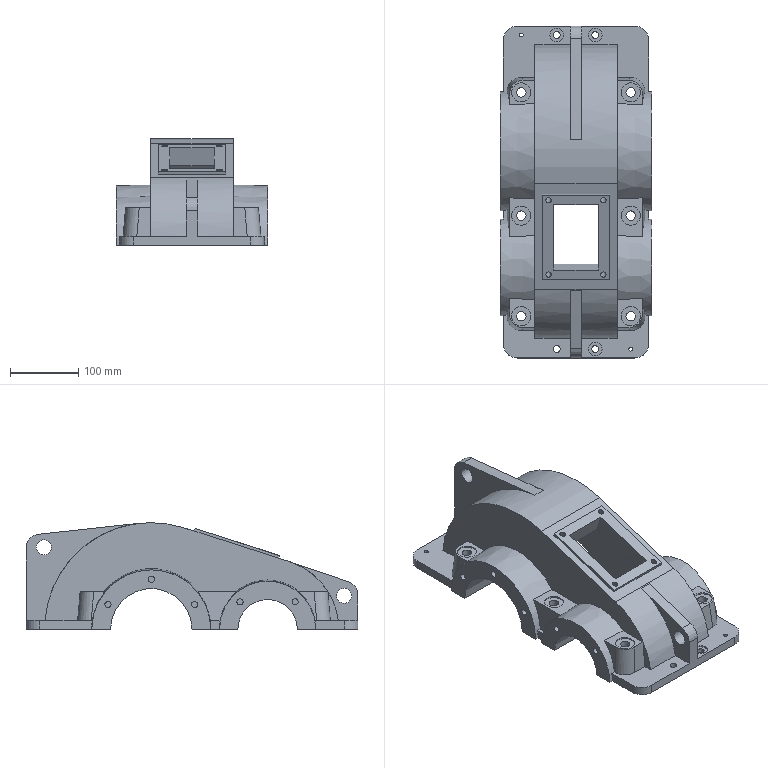Part | NX | features DATUM_CSYS 43, EXTRUDE 42, SKETCH 42, EXTRACT_DATUM_AXIS 38, EXTRACT_FACE 32, SIMPLE HOLE 23, EXTRACT_DATUM_PLANE 14, Instance Feature 13, DRAFT 9, EXTRACT_STRING 8, HOLE PACKAGE 8, FSET 6, Mirror Feature 5, BLEND 4, OFFSET_REGION 4, Pattern Feature 2 | 1 solid | 137 faces | box 222 x 485 x 156 mm | volume 3762838 mm3 | plane 78 | cylinder 55 | cone 4 | commonest cylinder face diameters 9 x10 40 x10 14 x6 28 x6 8 x4 10 x4